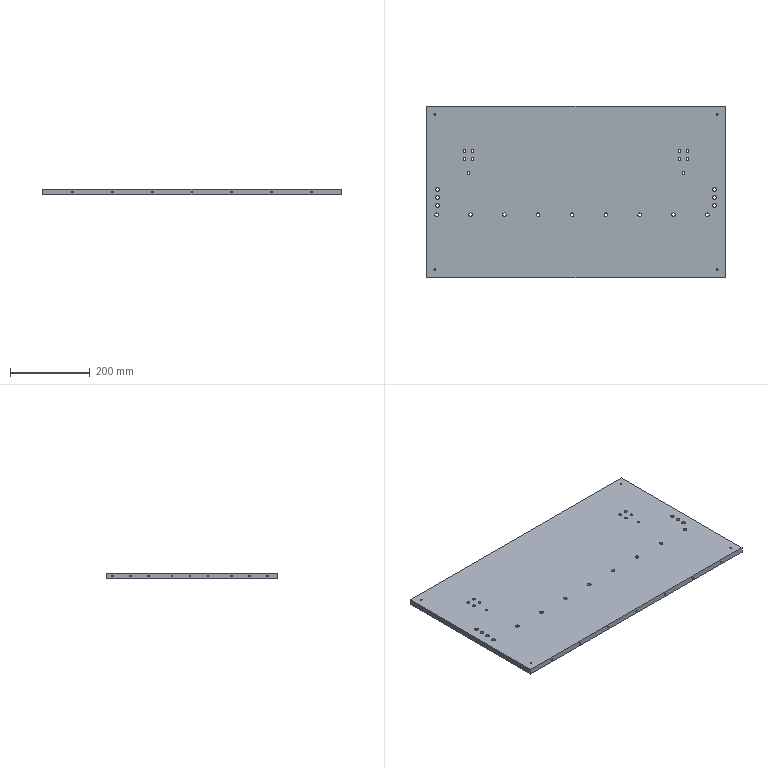Part | STEP file | MT-COMBO-119-S027 | 1 solid | 229 faces | box 750 x 430 x 14 mm | volume 4475183 mm3 | cylinder 148 | cone 60 | plane 21 | commonest cylinder face diameters 4.2 x68 9 x30 15 x30 6.8 x20